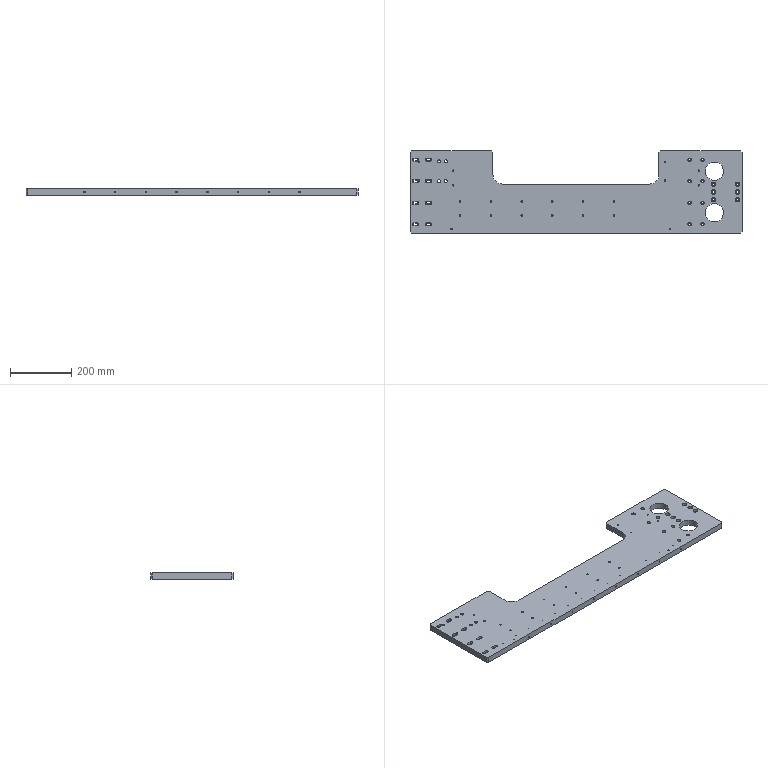Part | NX | 1 solid | 225 faces | box 1080 x 268 x 20 mm | volume 4450866 mm3 | cylinder 113 | plane 70 | cone 42 | commonest cylinder face diameters 5 x26 11 x25 7 x24 4.2 x16 9 x6 15 x6